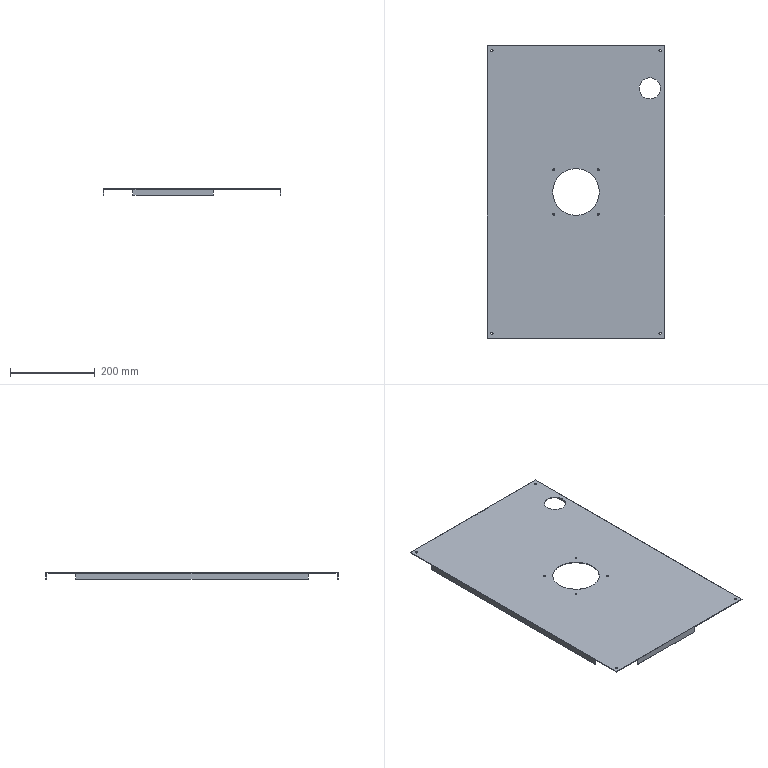Part | SolidWorks | features BaseBody 1 | 1 solid | 42 faces | box 418 x 688 x 15 mm | volume 443799 mm3 | plane 22 | cylinder 20 | commonest cylinder face diameters 4.2 x8 5.5 x8 50 x2 110 x2
STEP:
#1=CARTESIAN_POINT('',(49.25,332.999,-1.5));
#2=VERTEX_POINT('',#1);
#3=CARTESIAN_POINT('',(54.75,332.999,-1.5));
#4=VERTEX_POINT('',#3);
#5=CARTESIAN_POINT('',(52.,332.999,-1.5));
#6=DIRECTION('',(0.,0.,1.));
#7=DIRECTION('',(1.,0.,0.));
#8=AXIS2_PLACEMENT_3D('',#5,#6,#7);
#9=CIRCLE('',#8,2.75);
#10=EDGE_CURVE('',#2,#4,#9,.T.);
#11=ORIENTED_EDGE('',*,*,#10,.F.);
#12=CARTESIAN_POINT('',(49.25,332.999,0.));
#13=VERTEX_POINT('',#12);
#14=CARTESIAN_POINT('',(49.25,332.999,-15.));
#15=DIRECTION('',(0.,0.,1.));
#16=VECTOR('',#15,1000.);
#17=LINE('',#14,#16);
#18=EDGE_CURVE('',#2,#13,#17,.T.);
#19=ORIENTED_EDGE('',*,*,#18,.T.);
#20=CARTESIAN_POINT('',(54.75,332.999,0.));
#21=VERTEX_POINT('',#20);
#22=CARTESIAN_POINT('',(52.,332.999,0.));
#23=DIRECTION('',(0.,0.,-1.));
#24=DIRECTION('',(1.,0.,0.));
#25=AXIS2_PLACEMENT_3D('',#22,#23,#24);
#26=CIRCLE('',#25,2.75);
#27=EDGE_CURVE('',#21,#13,#26,.T.);
#28=ORIENTED_EDGE('',*,*,#27,.F.);
#29=CARTESIAN_POINT('',(54.75,332.999,-15.));
#30=DIRECTION('',(0.,0.,1.));
#31=VECTOR('',#30,1000.);
#32=LINE('',#29,#31);
#33=EDGE_CURVE('',#4,#21,#32,.T.);
#34=ORIENTED_EDGE('',*,*,#33,.F.);
#35=EDGE_LOOP('',(#11,#19,#28,#34));
#36=FACE_OUTER_BOUND('',#35,.T.);
#37=CARTESIAN_POINT('',(52.,332.999,-15.));
#38=DIRECTION('',(0.,0.,1.));
#39=DIRECTION('',(1.,0.,0.));
#40=AXIS2_PLACEMENT_3D('',#37,#38,#39);
#41=CYLINDRICAL_SURFACE('',#40,2.75);
#42=ADVANCED_FACE('',(#36),#41,.F.);
#43=CARTESIAN_POINT('',(445.249,333.,-1.5));
#44=VERTEX_POINT('',#43);
#45=CARTESIAN_POINT('',(450.749,333.,-1.5));
#46=VERTEX_POINT('',#45);
#47=CARTESIAN_POINT('',(447.999,333.,-1.5));
#48=DIRECTION('',(0.,0.,1.));
#49=DIRECTION('',(1.,0.,0.));
#50=AXIS2_PLACEMENT_3D('',#47,#48,#49);
#51=CIRCLE('',#50,2.75);
#52=EDGE_CURVE('',#44,#46,#51,.T.);
#53=ORIENTED_EDGE('',*,*,#52,.F.);
#54=CARTESIAN_POINT('',(445.249,333.,0.));
#55=VERTEX_POINT('',#54);
#56=CARTESIAN_POINT('',(445.249,333.,-15.));
#57=DIRECTION('',(0.,0.,1.));
#58=VECTOR('',#57,1000.);
#59=LINE('',#56,#58);
#60=EDGE_CURVE('',#44,#55,#59,.T.);
#61=ORIENTED_EDGE('',*,*,#60,.T.);
#62=CARTESIAN_POINT('',(450.749,333.,0.));
#63=VERTEX_POINT('',#62);
#64=CARTESIAN_POINT('',(447.999,333.,0.));
#65=DIRECTION('',(0.,0.,-1.));
#66=DIRECTION('',(1.,0.,0.));
#67=AXIS2_PLACEMENT_3D('',#64,#65,#66);
#68=CIRCLE('',#67,2.75);
#69=EDGE_CURVE('',#63,#55,#68,.T.);
#70=ORIENTED_EDGE('',*,*,#69,.F.);
#71=CARTESIAN_POINT('',(450.749,333.,-15.));
#72=DIRECTION('',(0.,0.,1.));
#73=VECTOR('',#72,1000.);
#74=LINE('',#71,#73);
#75=EDGE_CURVE('',#46,#63,#74,.T.);
#76=ORIENTED_EDGE('',*,*,#75,.F.);
#77=EDGE_LOOP('',(#53,#61,#70,#76));
#78=FACE_OUTER_BOUND('',#77,.T.);
#79=CARTESIAN_POINT('',(447.999,333.,-15.));
#80=DIRECTION('',(0.,0.,1.));
#81=DIRECTION('',(1.,0.,0.));
#82=AXIS2_PLACEMENT_3D('',#79,#80,#81);
#83=CYLINDRICAL_SURFACE('',#82,2.75);
#84=ADVANCED_FACE('',(#78),#83,.F.);
#85=CARTESIAN_POINT('',(49.251,-333.,-1.5));
#86=VERTEX_POINT('',#85);
#87=CARTESIAN_POINT('',(54.751,-333.,-1.5));
#88=VERTEX_POINT('',#87);
#89=CARTESIAN_POINT('',(52.001,-333.,-1.5));
#90=DIRECTION('',(0.,0.,1.));
#91=DIRECTION('',(1.,0.,0.));
#92=AXIS2_PLACEMENT_3D('',#89,#90,#91);
#93=CIRCLE('',#92,2.75);
#94=EDGE_CURVE('',#86,#88,#93,.T.);
#95=ORIENTED_EDGE('',*,*,#94,.F.);
#96=CARTESIAN_POINT('',(49.251,-333.,0.));
#97=VERTEX_POINT('',#96);
#98=CARTESIAN_POINT('',(49.251,-333.,-15.));
#99=DIRECTION('',(0.,0.,1.));
#100=VECTOR('',#99,1000.);
#101=LINE('',#98,#100);
#102=EDGE_CURVE('',#86,#97,#101,.T.);
#103=ORIENTED_EDGE('',*,*,#102,.T.);
#104=CARTESIAN_POINT('',(54.751,-333.,0.));
#105=VERTEX_POINT('',#104);
#106=CARTESIAN_POINT('',(52.001,-333.,0.));
#107=DIRECTION('',(0.,0.,-1.));
#108=DIRECTION('',(1.,0.,0.));
#109=AXIS2_PLACEMENT_3D('',#106,#107,#108);
#110=CIRCLE('',#109,2.75);
#111=EDGE_CURVE('',#105,#97,#110,.T.);
#112=ORIENTED_EDGE('',*,*,#111,.F.);
#113=CARTESIAN_POINT('',(54.751,-333.,-15.));
#114=DIRECTION('',(0.,0.,1.));
#115=VECTOR('',#114,1000.);
#116=LINE('',#113,#115);
#117=EDGE_CURVE('',#88,#105,#116,.T.);
#118=ORIENTED_EDGE('',*,*,#117,.F.);
#119=EDGE_LOOP('',(#95,#103,#112,#118));
#120=FACE_OUTER_BOUND('',#119,.T.);
#121=CARTESIAN_POINT('',(52.001,-333.,-15.));
#122=DIRECTION('',(0.,0.,1.));
#123=DIRECTION('',(1.,0.,0.));
#124=AXIS2_PLACEMENT_3D('',#121,#122,#123);
#125=CYLINDRICAL_SURFACE('',#124,2.75);
#126=ADVANCED_FACE('',(#120),#125,.F.);
#127=CARTESIAN_POINT('',(445.249,-333.,-1.5));
#128=VERTEX_POINT('',#127);
#129=CARTESIAN_POINT('',(450.749,-333.,-1.5));
#130=VERTEX_POINT('',#129);
#131=CARTESIAN_POINT('',(447.999,-333.,-1.5));
#132=DIRECTION('',(0.,0.,1.));
#133=DIRECTION('',(1.,0.,0.));
#134=AXIS2_PLACEMENT_3D('',#131,#132,#133);
#135=CIRCLE('',#134,2.75);
#136=EDGE_CURVE('',#128,#130,#135,.T.);
#137=ORIENTED_EDGE('',*,*,#136,.F.);
#138=CARTESIAN_POINT('',(445.249,-333.,0.));
#139=VERTEX_POINT('',#138);
#140=CARTESIAN_POINT('',(445.249,-333.,-15.));
#141=DIRECTION('',(0.,0.,1.));
#142=VECTOR('',#141,1000.);
#143=LINE('',#140,#142);
#144=EDGE_CURVE('',#128,#139,#143,.T.);
#145=ORIENTED_EDGE('',*,*,#144,.T.);
#146=CARTESIAN_POINT('',(450.749,-333.,0.));
#147=VERTEX_POINT('',#146);
#148=CARTESIAN_POINT('',(447.999,-333.,0.));
#149=DIRECTION('',(0.,0.,-1.));
#150=DIRECTION('',(1.,0.,0.));
#151=AXIS2_PLACEMENT_3D('',#148,#149,#150);
#152=CIRCLE('',#151,2.75);
#153=EDGE_CURVE('',#147,#139,#152,.T.);
#154=ORIENTED_EDGE('',*,*,#153,.F.);
#155=CARTESIAN_POINT('',(450.749,-333.,-15.));
#156=DIRECTION('',(0.,0.,1.));
#157=VECTOR('',#156,1000.);
#158=LINE('',#155,#157);
#159=EDGE_CURVE('',#130,#147,#158,.T.);
#160=ORIENTED_EDGE('',*,*,#159,.F.);
#161=EDGE_LOOP('',(#137,#145,#154,#160));
#162=FACE_OUTER_BOUND('',#161,.T.);
#163=CARTESIAN_POINT('',(447.999,-333.,-15.));
#164=DIRECTION('',(0.,0.,1.));
#165=DIRECTION('',(1.,0.,0.));
#166=AXIS2_PLACEMENT_3D('',#163,#164,#165);
#167=CYLINDRICAL_SURFACE('',#166,2.75);
#168=ADVANCED_FACE('',(#162),#167,.F.);
#169=CARTESIAN_POINT('',(399.,244.,-1.5));
#170=VERTEX_POINT('',#169);
#171=CARTESIAN_POINT('',(449.,244.,-1.5));
#172=VERTEX_POINT('',#171);
#173=CARTESIAN_POINT('',(424.,244.,-1.5));
#174=DIRECTION('',(0.,0.,1.));
#175=DIRECTION('',(1.,0.,0.));
#176=AXIS2_PLACEMENT_3D('',#173,#174,#175);
#177=CIRCLE('',#176,25.);
#178=EDGE_CURVE('',#170,#172,#177,.T.);
#179=ORIENTED_EDGE('',*,*,#178,.F.);
#180=CARTESIAN_POINT('',(399.,244.,0.));
#181=VERTEX_POINT('',#180);
#182=CARTESIAN_POINT('',(399.,244.,-15.));
#183=DIRECTION('',(0.,0.,1.));
#184=VECTOR('',#183,1000.);
#185=LINE('',#182,#184);
#186=EDGE_CURVE('',#170,#181,#185,.T.);
#187=ORIENTED_EDGE('',*,*,#186,.T.);
#188=CARTESIAN_POINT('',(449.,244.,0.));
#189=VERTEX_POINT('',#188);
#190=CARTESIAN_POINT('',(424.,244.,0.));
#191=DIRECTION('',(0.,0.,-1.));
#192=DIRECTION('',(1.,0.,0.));
#193=AXIS2_PLACEMENT_3D('',#190,#191,#192);
#194=CIRCLE('',#193,25.);
#195=EDGE_CURVE('',#189,#181,#194,.T.);
#196=ORIENTED_EDGE('',*,*,#195,.F.);
#197=CARTESIAN_POINT('',(449.,244.,-15.));
#198=DIRECTION('',(0.,0.,1.));
#199=VECTOR('',#198,1000.);
#200=LINE('',#197,#199);
#201=EDGE_CURVE('',#172,#189,#200,.T.);
#202=ORIENTED_EDGE('',*,*,#201,.F.);
#203=EDGE_LOOP('',(#179,#187,#196,#202));
#204=FACE_OUTER_BOUND('',#203,.T.);
#205=CARTESIAN_POINT('',(424.,244.,-15.));
#206=DIRECTION('',(0.,0.,1.));
#207=DIRECTION('',(1.,0.,0.));
#208=AXIS2_PLACEMENT_3D('',#205,#206,#207);
#209=CYLINDRICAL_SURFACE('',#208,25.);
#210=ADVANCED_FACE('',(#204),#209,.F.);
#211=CARTESIAN_POINT('',(195.,0.,-1.5));
#212=VERTEX_POINT('',#211);
#213=CARTESIAN_POINT('',(305.,0.,-1.5));
#214=VERTEX_POINT('',#213);
#215=CARTESIAN_POINT('',(250.,0.,-1.5));
#216=DIRECTION('',(0.,0.,1.));
#217=DIRECTION('',(1.,0.,0.));
#218=AXIS2_PLACEMENT_3D('',#215,#216,#217);
#219=CIRCLE('',#218,55.);
#220=EDGE_CURVE('',#212,#214,#219,.T.);
#221=ORIENTED_EDGE('',*,*,#220,.F.);
#222=CARTESIAN_POINT('',(195.,0.,0.));
#223=VERTEX_POINT('',#222);
#224=CARTESIAN_POINT('',(195.,0.,-15.001));
#225=DIRECTION('',(0.,0.,1.));
#226=VECTOR('',#225,1000.);
#227=LINE('',#224,#226);
#228=EDGE_CURVE('',#212,#223,#227,.T.);
#229=ORIENTED_EDGE('',*,*,#228,.T.);
#230=CARTESIAN_POINT('',(305.,0.,0.));
#231=VERTEX_POINT('',#230);
#232=CARTESIAN_POINT('',(250.,0.,0.));
#233=DIRECTION('',(0.,0.,-1.));
#234=DIRECTION('',(1.,0.,0.));
#235=AXIS2_PLACEMENT_3D('',#232,#233,#234);
#236=CIRCLE('',#235,55.);
#237=EDGE_CURVE('',#231,#223,#236,.T.);
#238=ORIENTED_EDGE('',*,*,#237,.F.);
#239=CARTESIAN_POINT('',(305.,0.,-15.001));
#240=DIRECTION('',(0.,0.,1.));
#241=VECTOR('',#240,1000.);
#242=LINE('',#239,#241);
#243=EDGE_CURVE('',#214,#231,#242,.T.);
#244=ORIENTED_EDGE('',*,*,#243,.F.);
#245=EDGE_LOOP('',(#221,#229,#238,#244));
#246=FACE_OUTER_BOUND('',#245,.T.);
#247=CARTESIAN_POINT('',(250.,0.,-15.001));
#248=DIRECTION('',(0.,0.,1.));
#249=DIRECTION('',(1.,0.,0.));
#250=AXIS2_PLACEMENT_3D('',#247,#248,#249);
#251=CYLINDRICAL_SURFACE('',#250,55.);
#252=ADVANCED_FACE('',(#246),#251,.F.);
#253=CARTESIAN_POINT('',(304.6,-52.5,0.));
#254=VERTEX_POINT('',#253);
#255=CARTESIAN_POINT('',(300.4,-52.5,0.));
#256=VERTEX_POINT('',#255);
#257=CARTESIAN_POINT('',(302.5,-52.5,0.));
#258=DIRECTION('',(0.,0.,-1.));
#259=DIRECTION('',(-1.,0.,0.));
#260=AXIS2_PLACEMENT_3D('',#257,#258,#259);
#261=CIRCLE('',#260,2.1);
#262=EDGE_CURVE('',#254,#256,#261,.T.);
#263=ORIENTED_EDGE('',*,*,#262,.F.);
#264=CARTESIAN_POINT('',(304.6,-52.5,-1.5));
#265=VERTEX_POINT('',#264);
#266=CARTESIAN_POINT('',(304.6,-52.5,-1.5));
#267=DIRECTION('',(0.,0.,-1.));
#268=VECTOR('',#267,1000.);
#269=LINE('',#266,#268);
#270=EDGE_CURVE('',#254,#265,#269,.T.);
#271=ORIENTED_EDGE('',*,*,#270,.T.);
#272=CARTESIAN_POINT('',(300.4,-52.5,-1.5));
#273=VERTEX_POINT('',#272);
#274=CARTESIAN_POINT('',(302.5,-52.5,-1.5));
#275=DIRECTION('',(0.,0.,1.));
#276=DIRECTION('',(-1.,0.,0.));
#277=AXIS2_PLACEMENT_3D('',#274,#275,#276);
#278=CIRCLE('',#277,2.1);
#279=EDGE_CURVE('',#273,#265,#278,.T.);
#280=ORIENTED_EDGE('',*,*,#279,.F.);
#281=CARTESIAN_POINT('',(300.4,-52.5,-1.5));
#282=DIRECTION('',(0.,0.,-1.));
#283=VECTOR('',#282,1000.);
#284=LINE('',#281,#283);
#285=EDGE_CURVE('',#256,#273,#284,.T.);
#286=ORIENTED_EDGE('',*,*,#285,.F.);
#287=EDGE_LOOP('',(#263,#271,#280,#286));
#288=FACE_OUTER_BOUND('',#287,.T.);
#289=CARTESIAN_POINT('',(302.5,-52.5,-1.5));
#290=DIRECTION('',(0.,0.,-1.));
#291=DIRECTION('',(-1.,0.,0.));
#292=AXIS2_PLACEMENT_3D('',#289,#290,#291);
#293=CYLINDRICAL_SURFACE('',#292,2.1);
#294=ADVANCED_FACE('',(#288),#293,.F.);
#295=CARTESIAN_POINT('',(199.6,-52.5,0.));
#296=VERTEX_POINT('',#295);
#297=CARTESIAN_POINT('',(195.4,-52.5,0.));
#298=VERTEX_POINT('',#297);
#299=CARTESIAN_POINT('',(197.5,-52.5,0.));
#300=DIRECTION('',(0.,0.,-1.));
#301=DIRECTION('',(-1.,0.,0.));
#302=AXIS2_PLACEMENT_3D('',#299,#300,#301);
#303=CIRCLE('',#302,2.1);
#304=EDGE_CURVE('',#296,#298,#303,.T.);
#305=ORIENTED_EDGE('',*,*,#304,.F.);
#306=CARTESIAN_POINT('',(199.6,-52.5,-1.5));
#307=VERTEX_POINT('',#306);
#308=CARTESIAN_POINT('',(199.6,-52.5,-1.5));
#309=DIRECTION('',(0.,0.,-1.));
#310=VECTOR('',#309,1000.);
#311=LINE('',#308,#310);
#312=EDGE_CURVE('',#296,#307,#311,.T.);
#313=ORIENTED_EDGE('',*,*,#312,.T.);
#314=CARTESIAN_POINT('',(195.4,-52.5,-1.5));
#315=VERTEX_POINT('',#314);
#316=CARTESIAN_POINT('',(197.5,-52.5,-1.5));
#317=DIRECTION('',(0.,0.,1.));
#318=DIRECTION('',(-1.,0.,0.));
#319=AXIS2_PLACEMENT_3D('',#316,#317,#318);
#320=CIRCLE('',#319,2.1);
#321=EDGE_CURVE('',#315,#307,#320,.T.);
#322=ORIENTED_EDGE('',*,*,#321,.F.);
#323=CARTESIAN_POINT('',(195.4,-52.5,-1.5));
#324=DIRECTION('',(0.,0.,-1.));
#325=VECTOR('',#324,1000.);
#326=LINE('',#323,#325);
#327=EDGE_CURVE('',#298,#315,#326,.T.);
#328=ORIENTED_EDGE('',*,*,#327,.F.);
#329=EDGE_LOOP('',(#305,#313,#322,#328));
#330=FACE_OUTER_BOUND('',#329,.T.);
#331=CARTESIAN_POINT('',(197.5,-52.5,-1.5));
#332=DIRECTION('',(0.,0.,-1.));
#333=DIRECTION('',(-1.,0.,0.));
#334=AXIS2_PLACEMENT_3D('',#331,#332,#333);
#335=CYLINDRICAL_SURFACE('',#334,2.1);
#336=ADVANCED_FACE('',(#330),#335,.F.);
#337=CARTESIAN_POINT('',(199.6,52.5,0.));
#338=VERTEX_POINT('',#337);
#339=CARTESIAN_POINT('',(195.4,52.5,0.));
#340=VERTEX_POINT('',#339);
#341=CARTESIAN_POINT('',(197.5,52.5,0.));
#342=DIRECTION('',(0.,0.,-1.));
#343=DIRECTION('',(-1.,0.,0.));
#344=AXIS2_PLACEMENT_3D('',#341,#342,#343);
#345=CIRCLE('',#344,2.1);
#346=EDGE_CURVE('',#338,#340,#345,.T.);
#347=ORIENTED_EDGE('',*,*,#346,.F.);
#348=CARTESIAN_POINT('',(199.6,52.5,-1.5));
#349=VERTEX_POINT('',#348);
#350=CARTESIAN_POINT('',(199.6,52.5,-1.5));
#351=DIRECTION('',(0.,0.,-1.));
#352=VECTOR('',#351,1000.);
#353=LINE('',#350,#352);
#354=EDGE_CURVE('',#338,#349,#353,.T.);
#355=ORIENTED_EDGE('',*,*,#354,.T.);
#356=CARTESIAN_POINT('',(195.4,52.5,-1.5));
#357=VERTEX_POINT('',#356);
#358=CARTESIAN_POINT('',(197.5,52.5,-1.5));
#359=DIRECTION('',(0.,0.,1.));
#360=DIRECTION('',(-1.,0.,0.));
#361=AXIS2_PLACEMENT_3D('',#358,#359,#360);
#362=CIRCLE('',#361,2.1);
#363=EDGE_CURVE('',#357,#349,#362,.T.);
#364=ORIENTED_EDGE('',*,*,#363,.F.);
#365=CARTESIAN_POINT('',(195.4,52.5,-1.5));
#366=DIRECTION('',(0.,0.,-1.));
#367=VECTOR('',#366,1000.);
#368=LINE('',#365,#367);
#369=EDGE_CURVE('',#340,#357,#368,.T.);
#370=ORIENTED_EDGE('',*,*,#369,.F.);
#371=EDGE_LOOP('',(#347,#355,#364,#370));
#372=FACE_OUTER_BOUND('',#371,.T.);
#373=CARTESIAN_POINT('',(197.5,52.5,-1.5));
#374=DIRECTION('',(0.,0.,-1.));
#375=DIRECTION('',(-1.,0.,0.));
#376=AXIS2_PLACEMENT_3D('',#373,#374,#375);
#377=CYLINDRICAL_SURFACE('',#376,2.1);
#378=ADVANCED_FACE('',(#372),#377,.F.);
#379=CARTESIAN_POINT('',(304.6,52.5,0.));
#380=VERTEX_POINT('',#379);
#381=CARTESIAN_POINT('',(300.4,52.5,0.));
#382=VERTEX_POINT('',#381);
#383=CARTESIAN_POINT('',(302.5,52.5,0.));
#384=DIRECTION('',(0.,0.,-1.));
#385=DIRECTION('',(-1.,0.,0.));
#386=AXIS2_PLACEMENT_3D('',#383,#384,#385);
#387=CIRCLE('',#386,2.1);
#388=EDGE_CURVE('',#380,#382,#387,.T.);
#389=ORIENTED_EDGE('',*,*,#388,.F.);
#390=CARTESIAN_POINT('',(304.6,52.5,-1.5));
#391=VERTEX_POINT('',#390);
#392=CARTESIAN_POINT('',(304.6,52.5,-1.5));
#393=DIRECTION('',(0.,0.,-1.));
#394=VECTOR('',#393,1000.);
#395=LINE('',#392,#394);
#396=EDGE_CURVE('',#380,#391,#395,.T.);
#397=ORIENTED_EDGE('',*,*,#396,.T.);
#398=CARTESIAN_POINT('',(300.4,52.5,-1.5));
#399=VERTEX_POINT('',#398);
#400=CARTESIAN_POINT('',(302.5,52.5,-1.5));
#401=DIRECTION('',(0.,0.,1.));
#402=DIRECTION('',(-1.,0.,0.));
#403=AXIS2_PLACEMENT_3D('',#400,#401,#402);
#404=CIRCLE('',#403,2.1);
#405=EDGE_CURVE('',#399,#391,#404,.T.);
#406=ORIENTED_EDGE('',*,*,#405,.F.);
#407=CARTESIAN_POINT('',(300.4,52.5,-1.5));
#408=DIRECTION('',(0.,0.,-1.));
#409=VECTOR('',#408,1000.);
#410=LINE('',#407,#409);
#411=EDGE_CURVE('',#382,#399,#410,.T.);
#412=ORIENTED_EDGE('',*,*,#411,.F.);
#413=EDGE_LOOP('',(#389,#397,#406,#412));
#414=FACE_OUTER_BOUND('',#413,.T.);
#415=CARTESIAN_POINT('',(302.5,52.5,-1.5));
#416=DIRECTION('',(0.,0.,-1.));
#417=DIRECTION('',(-1.,0.,0.));
#418=AXIS2_PLACEMENT_3D('',#415,#416,#417);
#419=CYLINDRICAL_SURFACE('',#418,2.1);
#420=ADVANCED_FACE('',(#414),#419,.F.);
#421=CARTESIAN_POINT('',(459.,-344.,0.));
#422=VERTEX_POINT('',#421);
#423=CARTESIAN_POINT('',(459.,344.,0.));
#424=VERTEX_POINT('',#423);
#425=CARTESIAN_POINT('',(459.,0.,0.));
#426=DIRECTION('',(0.,1.,0.));
#427=VECTOR('',#426,1000.);
#428=LINE('',#425,#427);
#429=EDGE_CURVE('',#422,#424,#428,.T.);
#430=ORIENTED_EDGE('',*,*,#429,.T.);
#431=CARTESIAN_POINT('',(41.,344.,0.));
#432=VERTEX_POINT('',#431);
#433=CARTESIAN_POINT('',(0.,344.,0.));
#434=DIRECTION('',(-1.,0.,0.));
#435=VECTOR('',#434,1000.);
#436=LINE('',#433,#435);
#437=EDGE_CURVE('',#424,#432,#436,.T.);
#438=ORIENTED_EDGE('',*,*,#437,.T.);
#439=CARTESIAN_POINT('',(41.,-344.,0.));
#440=VERTEX_POINT('',#439);
#441=CARTESIAN_POINT('',(41.,0.,0.));
#442=DIRECTION('',(0.,-1.,0.));
#443=VECTOR('',#442,1000.);
#444=LINE('',#441,#443);
#445=EDGE_CURVE('',#432,#440,#444,.T.);
#446=ORIENTED_EDGE('',*,*,#445,.T.);
#447=CARTESIAN_POINT('',(0.,-344.,0.));
#448=DIRECTION('',(1.,0.,0.));
#449=VECTOR('',#448,1000.);
#450=LINE('',#447,#449);
#451=EDGE_CURVE('',#440,#422,#450,.T.);
#452=ORIENTED_EDGE('',*,*,#451,.T.);
#453=EDGE_LOOP('',(#430,#438,#446,#452));
#454=FACE_OUTER_BOUND('',#453,.T.);
#455=ORIENTED_EDGE('',*,*,#27,.T.);
#456=CARTESIAN_POINT('',(52.,332.999,0.));
#457=DIRECTION('',(0.,0.,-1.));
#458=DIRECTION('',(1.,0.,0.));
#459=AXIS2_PLACEMENT_3D('',#456,#457,#458);
#460=CIRCLE('',#459,2.75);
#461=EDGE_CURVE('',#13,#21,#460,.T.);
#462=ORIENTED_EDGE('',*,*,#461,.T.);
#463=EDGE_LOOP('',(#455,#462));
#464=FACE_BOUND('',#463,.T.);
#465=ORIENTED_EDGE('',*,*,#69,.T.);
#466=CARTESIAN_POINT('',(447.999,333.,0.));
#467=DIRECTION('',(0.,0.,-1.));
#468=DIRECTION('',(1.,0.,0.));
#469=AXIS2_PLACEMENT_3D('',#466,#467,#468);
#470=CIRCLE('',#469,2.75);
#471=EDGE_CURVE('',#55,#63,#470,.T.);
#472=ORIENTED_EDGE('',*,*,#471,.T.);
#473=EDGE_LOOP('',(#465,#472));
#474=FACE_BOUND('',#473,.T.);
#475=ORIENTED_EDGE('',*,*,#111,.T.);
#476=CARTESIAN_POINT('',(52.001,-333.,0.));
#477=DIRECTION('',(0.,0.,-1.));
#478=DIRECTION('',(1.,0.,0.));
#479=AXIS2_PLACEMENT_3D('',#476,#477,#478);
#480=CIRCLE('',#479,2.75);
#481=EDGE_CURVE('',#97,#105,#480,.T.);
#482=ORIENTED_EDGE('',*,*,#481,.T.);
#483=EDGE_LOOP('',(#475,#482));
#484=FACE_BOUND('',#483,.T.);
#485=ORIENTED_EDGE('',*,*,#153,.T.);
#486=CARTESIAN_POINT('',(447.999,-333.,0.));
#487=DIRECTION('',(0.,0.,-1.));
#488=DIRECTION('',(1.,0.,0.));
#489=AXIS2_PLACEMENT_3D('',#486,#487,#488);
#490=CIRCLE('',#489,2.75);
#491=EDGE_CURVE('',#139,#147,#490,.T.);
#492=ORIENTED_EDGE('',*,*,#491,.T.);
#493=EDGE_LOOP('',(#485,#492));
#494=FACE_BOUND('',#493,.T.);
#495=ORIENTED_EDGE('',*,*,#195,.T.);
#496=CARTESIAN_POINT('',(424.,244.,0.));
#497=DIRECTION('',(0.,0.,-1.));
#498=DIRECTION('',(1.,0.,0.));
#499=AXIS2_PLACEMENT_3D('',#496,#497,#498);
#500=CIRCLE('',#499,25.);
#501=EDGE_CURVE('',#181,#189,#500,.T.);
#502=ORIENTED_EDGE('',*,*,#501,.T.);
#503=EDGE_LOOP('',(#495,#502));
#504=FACE_BOUND('',#503,.T.);
#505=ORIENTED_EDGE('',*,*,#237,.T.);
#506=CARTESIAN_POINT('',(250.,0.,0.));
#507=DIRECTION('',(0.,0.,-1.));
#508=DIRECTION('',(1.,0.,0.));
#509=AXIS2_PLACEMENT_3D('',#506,#507,#508);
#510=CIRCLE('',#509,55.);
#511=EDGE_CURVE('',#223,#231,#510,.T.);
#512=ORIENTED_EDGE('',*,*,#511,.T.);
#513=EDGE_LOOP('',(#505,#512));
#514=FACE_BOUND('',#513,.T.);
#515=CARTESIAN_POINT('',(302.5,-52.5,0.));
#516=DIRECTION('',(0.,0.,-1.));
#517=DIRECTION('',(-1.,0.,0.));
#518=AXIS2_PLACEMENT_3D('',#515,#516,#517);
#519=CIRCLE('',#518,2.1);
#520=EDGE_CURVE('',#256,#254,#519,.T.);
#521=ORIENTED_EDGE('',*,*,#520,.T.);
#522=ORIENTED_EDGE('',*,*,#262,.T.);
#523=EDGE_LOOP('',(#521,#522));
#524=FACE_BOUND('',#523,.T.);
#525=CARTESIAN_POINT('',(197.5,-52.5,0.));
#526=DIRECTION('',(0.,0.,-1.));
#527=DIRECTION('',(-1.,0.,0.));
#528=AXIS2_PLACEMENT_3D('',#525,#526,#527);
#529=CIRCLE('',#528,2.1);
#530=EDGE_CURVE('',#298,#296,#529,.T.);
#531=ORIENTED_EDGE('',*,*,#530,.T.);
#532=ORIENTED_EDGE('',*,*,#304,.T.);
#533=EDGE_LOOP('',(#531,#532));
#534=FACE_BOUND('',#533,.T.);
#535=CARTESIAN_POINT('',(197.5,52.5,0.));
#536=DIRECTION('',(0.,0.,-1.));
#537=DIRECTION('',(-1.,0.,0.));
#538=AXIS2_PLACEMENT_3D('',#535,#536,#537);
#539=CIRCLE('',#538,2.1);
#540=EDGE_CURVE('',#340,#338,#539,.T.);
#541=ORIENTED_EDGE('',*,*,#540,.T.);
#542=ORIENTED_EDGE('',*,*,#346,.T.);
#543=EDGE_LOOP('',(#541,#542));
#544=FACE_BOUND('',#543,.T.);
#545=CARTESIAN_POINT('',(302.5,52.5,0.));
#546=DIRECTION('',(0.,0.,-1.));
#547=DIRECTION('',(-1.,0.,0.));
#548=AXIS2_PLACEMENT_3D('',#545,#546,#547);
#549=CIRCLE('',#548,2.1);
#550=EDGE_CURVE('',#382,#380,#549,.T.);
#551=ORIENTED_EDGE('',*,*,#550,.T.);
#552=ORIENTED_EDGE('',*,*,#388,.T.);
#553=EDGE_LOOP('',(#551,#552));
#554=FACE_BOUND('',#553,.T.);
#555=CARTESIAN_POINT('',(0.,0.,0.));
#556=DIRECTION('',(0.,0.,1.));
#557=DIRECTION('',(1.,0.,0.));
#558=AXIS2_PLACEMENT_3D('',#555,#556,#557);
#559=PLANE('',#558);
#560=ADVANCED_FACE('',(#454,#464,#474,#484,#494,#504,#514,#524,#534,#544,#554),#559,.T.);
#561=ORIENTED_EDGE('',*,*,#437,.F.);
#562=CARTESIAN_POINT('',(459.,344.,-1.5));
#563=VERTEX_POINT('',#562);
#564=CARTESIAN_POINT('',(459.,344.,-15.));
#565=DIRECTION('',(0.,0.,-1.));
#566=VECTOR('',#565,1000.);
#567=LINE('',#564,#566);
#568=EDGE_CURVE('',#424,#563,#567,.T.);
#569=ORIENTED_EDGE('',*,*,#568,.T.);
#570=CARTESIAN_POINT('',(300.,344.,-1.5));
#571=VERTEX_POINT('',#570);
#572=CARTESIAN_POINT('',(41.,344.,-1.5));
#573=DIRECTION('',(-1.,0.,0.));
#574=VECTOR('',#573,1000.);
#575=LINE('',#572,#574);
#576=EDGE_CURVE('',#563,#571,#575,.T.);
#577=ORIENTED_EDGE('',*,*,#576,.T.);
#578=CARTESIAN_POINT('',(300.,344.,-15.));
#579=VERTEX_POINT('',#578);
#580=CARTESIAN_POINT('',(300.,344.,-15.));
#581=DIRECTION('',(0.,0.,-1.));
#582=VECTOR('',#581,1000.);
#583=LINE('',#580,#582);
#584=EDGE_CURVE('',#571,#579,#583,.T.);
#585=ORIENTED_EDGE('',*,*,#584,.T.);
#586=CARTESIAN_POINT('',(111.,344.,-15.));
#587=VERTEX_POINT('',#586);
#588=CARTESIAN_POINT('',(41.,344.,-15.));
#589=DIRECTION('',(-1.,0.,0.));
#590=VECTOR('',#589,1000.);
#591=LINE('',#588,#590);
#592=EDGE_CURVE('',#579,#587,#591,.T.);
#593=ORIENTED_EDGE('',*,*,#592,.T.);
#594=CARTESIAN_POINT('',(111.,344.,-1.5));
#595=VERTEX_POINT('',#594);
#596=CARTESIAN_POINT('',(111.,344.,-15.));
#597=DIRECTION('',(0.,0.,1.));
#598=VECTOR('',#597,1000.);
#599=LINE('',#596,#598);
#600=EDGE_CURVE('',#587,#595,#599,.T.);
#601=ORIENTED_EDGE('',*,*,#600,.T.);
#602=CARTESIAN_POINT('',(41.,344.,-1.5));
#603=VERTEX_POINT('',#602);
#604=CARTESIAN_POINT('',(41.,344.,-1.5));
#605=DIRECTION('',(-1.,0.,0.));
#606=VECTOR('',#605,1000.);
#607=LINE('',#604,#606);
#608=EDGE_CURVE('',#595,#603,#607,.T.);
#609=ORIENTED_EDGE('',*,*,#608,.T.);
#610=CARTESIAN_POINT('',(41.,344.,-15.));
#611=DIRECTION('',(0.,0.,1.));
#612=VECTOR('',#611,1000.);
#613=LINE('',#610,#612);
#614=EDGE_CURVE('',#603,#432,#613,.T.);
#615=ORIENTED_EDGE('',*,*,#614,.T.);
#616=EDGE_LOOP('',(#561,#569,#577,#585,#593,#601,#609,#615));
#617=FACE_OUTER_BOUND('',#616,.T.);
#618=CARTESIAN_POINT('',(41.,344.,-15.));
#619=DIRECTION('',(0.,1.,0.));
#620=DIRECTION('',(0.,0.,1.));
#621=AXIS2_PLACEMENT_3D('',#618,#619,#620);
#622=PLANE('',#621);
#623=ADVANCED_FACE('',(#617),#622,.T.);
#624=ORIENTED_EDGE('',*,*,#429,.F.);
#625=CARTESIAN_POINT('',(459.,-344.,-1.5));
#626=VERTEX_POINT('',#625);
#627=CARTESIAN_POINT('',(459.,-344.,-15.));
#628=DIRECTION('',(0.,0.,-1.));
#629=VECTOR('',#628,1000.);
#630=LINE('',#627,#629);
#631=EDGE_CURVE('',#422,#626,#630,.T.);
#632=ORIENTED_EDGE('',*,*,#631,.T.);
#633=CARTESIAN_POINT('',(459.,-274.,-1.5));
#634=VERTEX_POINT('',#633);
#635=CARTESIAN_POINT('',(459.,344.,-1.5));
#636=DIRECTION('',(0.,1.,0.));
#637=VECTOR('',#636,1000.);
#638=LINE('',#635,#637);
#639=EDGE_CURVE('',#626,#634,#638,.T.);
#640=ORIENTED_EDGE('',*,*,#639,.T.);
#641=CARTESIAN_POINT('',(459.,-274.,-15.));
#642=VERTEX_POINT('',#641);
#643=CARTESIAN_POINT('',(459.,-274.,-15.));
#644=DIRECTION('',(0.,0.,-1.));
#645=VECTOR('',#644,1000.);
#646=LINE('',#643,#645);
#647=EDGE_CURVE('',#634,#642,#646,.T.);
#648=ORIENTED_EDGE('',*,*,#647,.T.);
#649=CARTESIAN_POINT('',(459.,274.,-15.));
#650=VERTEX_POINT('',#649);
#651=CARTESIAN_POINT('',(459.,344.,-15.));
#652=DIRECTION('',(0.,1.,0.));
#653=VECTOR('',#652,1000.);
#654=LINE('',#651,#653);
#655=EDGE_CURVE('',#642,#650,#654,.T.);
#656=ORIENTED_EDGE('',*,*,#655,.T.);
#657=CARTESIAN_POINT('',(459.,274.,-1.5));
#658=VERTEX_POINT('',#657);
#659=CARTESIAN_POINT('',(459.,274.,-15.));
#660=DIRECTION('',(0.,0.,1.));
#661=VECTOR('',#660,1000.);
#662=LINE('',#659,#661);
#663=EDGE_CURVE('',#650,#658,#662,.T.);
#664=ORIENTED_EDGE('',*,*,#663,.T.);
#665=CARTESIAN_POINT('',(459.,344.,-1.5));
#666=DIRECTION('',(0.,1.,0.));
#667=VECTOR('',#666,1000.);
#668=LINE('',#665,#667);
#669=EDGE_CURVE('',#658,#563,#668,.T.);
#670=ORIENTED_EDGE('',*,*,#669,.T.);
#671=ORIENTED_EDGE('',*,*,#568,.F.);
#672=EDGE_LOOP('',(#624,#632,#640,#648,#656,#664,#670,#671));
#673=FACE_OUTER_BOUND('',#672,.T.);
#674=CARTESIAN_POINT('',(459.,344.,-15.));
#675=DIRECTION('',(1.,0.,0.));
#676=DIRECTION('',(0.,1.,0.));
#677=AXIS2_PLACEMENT_3D('',#674,#675,#676);
#678=PLANE('',#677);
#679=ADVANCED_FACE('',(#673),#678,.T.);
#680=CARTESIAN_POINT('',(41.,-344.,-1.5));
#681=VERTEX_POINT('',#680);
#682=CARTESIAN_POINT('',(111.,-344.,-1.5));
#683=VERTEX_POINT('',#682);
#684=CARTESIAN_POINT('',(41.,-344.,-1.5));
#685=DIRECTION('',(1.,0.,0.));
#686=VECTOR('',#685,1000.);
#687=LINE('',#684,#686);
#688=EDGE_CURVE('',#681,#683,#687,.T.);
#689=ORIENTED_EDGE('',*,*,#688,.T.);
#690=CARTESIAN_POINT('',(111.,-344.,-15.));
#691=VERTEX_POINT('',#690);
#692=CARTESIAN_POINT('',(111.,-344.,-15.));
#693=DIRECTION('',(0.,0.,-1.));
#694=VECTOR('',#693,1000.);
#695=LINE('',#692,#694);
#696=EDGE_CURVE('',#683,#691,#695,.T.);
#697=ORIENTED_EDGE('',*,*,#696,.T.);
#698=CARTESIAN_POINT('',(300.,-344.,-15.));
#699=VERTEX_POINT('',#698);
#700=CARTESIAN_POINT('',(41.,-344.,-15.));
#701=DIRECTION('',(1.,0.,0.));
#702=VECTOR('',#701,1000.);
#703=LINE('',#700,#702);
#704=EDGE_CURVE('',#691,#699,#703,.T.);
#705=ORIENTED_EDGE('',*,*,#704,.T.);
#706=CARTESIAN_POINT('',(300.,-344.,-1.5));
#707=VERTEX_POINT('',#706);
#708=CARTESIAN_POINT('',(300.,-344.,-15.));
#709=DIRECTION('',(0.,0.,1.));
#710=VECTOR('',#709,1000.);
#711=LINE('',#708,#710);
#712=EDGE_CURVE('',#699,#707,#711,.T.);
#713=ORIENTED_EDGE('',*,*,#712,.T.);
#714=CARTESIAN_POINT('',(41.,-344.,-1.5));
#715=DIRECTION('',(1.,0.,0.));
#716=VECTOR('',#715,1000.);
#717=LINE('',#714,#716);
#718=EDGE_CURVE('',#707,#626,#717,.T.);
#719=ORIENTED_EDGE('',*,*,#718,.T.);
#720=ORIENTED_EDGE('',*,*,#631,.F.);
#721=ORIENTED_EDGE('',*,*,#451,.F.);
#722=CARTESIAN_POINT('',(41.,-344.,-15.));
#723=DIRECTION('',(0.,0.,-1.));
#724=VECTOR('',#723,1000.);
#725=LINE('',#722,#724);
#726=EDGE_CURVE('',#440,#681,#725,.T.);
#727=ORIENTED_EDGE('',*,*,#726,.T.);
#728=EDGE_LOOP('',(#689,#697,#705,#713,#719,#720,#721,#727));
#729=FACE_OUTER_BOUND('',#728,.T.);
#730=CARTESIAN_POINT('',(41.,-344.,-15.));
#731=DIRECTION('',(0.,-1.,0.));
#732=DIRECTION('',(0.,0.,-1.));
#733=AXIS2_PLACEMENT_3D('',#730,#731,#732);
#734=PLANE('',#733);
#735=ADVANCED_FACE('',(#729),#734,.T.);
#736=CARTESIAN_POINT('',(41.,274.,-1.5));
#737=VERTEX_POINT('',#736);
#738=CARTESIAN_POINT('',(41.,344.,-1.5));
#739=DIRECTION('',(0.,-1.,0.));
#740=VECTOR('',#739,1000.);
#741=LINE('',#738,#740);
#742=EDGE_CURVE('',#603,#737,#741,.T.);
#743=ORIENTED_EDGE('',*,*,#742,.T.);
#744=CARTESIAN_POINT('',(41.,274.,-15.));
#745=VERTEX_POINT('',#744);
#746=CARTESIAN_POINT('',(41.,274.,-15.));
#747=DIRECTION('',(0.,0.,-1.));
#748=VECTOR('',#747,1000.);
#749=LINE('',#746,#748);
#750=EDGE_CURVE('',#737,#745,#749,.T.);
#751=ORIENTED_EDGE('',*,*,#750,.T.);
#752=CARTESIAN_POINT('',(41.,-274.,-15.));
#753=VERTEX_POINT('',#752);
#754=CARTESIAN_POINT('',(41.,344.,-15.));
#755=DIRECTION('',(0.,-1.,0.));
#756=VECTOR('',#755,1000.);
#757=LINE('',#754,#756);
#758=EDGE_CURVE('',#745,#753,#757,.T.);
#759=ORIENTED_EDGE('',*,*,#758,.T.);
#760=CARTESIAN_POINT('',(41.,-274.,-1.5));
#761=VERTEX_POINT('',#760);
#762=CARTESIAN_POINT('',(41.,-274.,-15.));
#763=DIRECTION('',(0.,0.,1.));
#764=VECTOR('',#763,1000.);
#765=LINE('',#762,#764);
#766=EDGE_CURVE('',#753,#761,#765,.T.);
#767=ORIENTED_EDGE('',*,*,#766,.T.);
#768=CARTESIAN_POINT('',(41.,344.,-1.5));
#769=DIRECTION('',(0.,-1.,0.));
#770=VECTOR('',#769,1000.);
#771=LINE('',#768,#770);
#772=EDGE_CURVE('',#761,#681,#771,.T.);
#773=ORIENTED_EDGE('',*,*,#772,.T.);
#774=ORIENTED_EDGE('',*,*,#726,.F.);
#775=ORIENTED_EDGE('',*,*,#445,.F.);
#776=ORIENTED_EDGE('',*,*,#614,.F.);
#777=EDGE_LOOP('',(#743,#751,#759,#767,#773,#774,#775,#776));
#778=FACE_OUTER_BOUND('',#777,.T.);
#779=CARTESIAN_POINT('',(41.,344.,-15.));
#780=DIRECTION('',(-1.,0.,0.));
#781=DIRECTION('',(0.,-1.,0.));
#782=AXIS2_PLACEMENT_3D('',#779,#780,#781);
#783=PLANE('',#782);
#784=ADVANCED_FACE('',(#778),#783,.T.);
#785=ORIENTED_EDGE('',*,*,#18,.F.);
#786=CARTESIAN_POINT('',(52.,332.999,-1.5));
#787=DIRECTION('',(0.,0.,1.));
#788=DIRECTION('',(1.,0.,0.));
#789=AXIS2_PLACEMENT_3D('',#786,#787,#788);
#790=CIRCLE('',#789,2.75);
#791=EDGE_CURVE('',#4,#2,#790,.T.);
#792=ORIENTED_EDGE('',*,*,#791,.F.);
#793=ORIENTED_EDGE('',*,*,#33,.T.);
#794=ORIENTED_EDGE('',*,*,#461,.F.);
#795=EDGE_LOOP('',(#785,#792,#793,#794));
#796=FACE_OUTER_BOUND('',#795,.T.);
#797=CARTESIAN_POINT('',(52.,332.999,-15.));
#798=DIRECTION('',(0.,0.,1.));
#799=DIRECTION('',(1.,0.,0.));
#800=AXIS2_PLACEMENT_3D('',#797,#798,#799);
#801=CYLINDRICAL_SURFACE('',#800,2.75);
#802=ADVANCED_FACE('',(#796),#801,.F.);
#803=ORIENTED_EDGE('',*,*,#60,.F.);
#804=CARTESIAN_POINT('',(447.999,333.,-1.5));
#805=DIRECTION('',(0.,0.,1.));
#806=DIRECTION('',(1.,0.,0.));
#807=AXIS2_PLACEMENT_3D('',#804,#805,#806);
#808=CIRCLE('',#807,2.75);
#809=EDGE_CURVE('',#46,#44,#808,.T.);
#810=ORIENTED_EDGE('',*,*,#809,.F.);
#811=ORIENTED_EDGE('',*,*,#75,.T.);
#812=ORIENTED_EDGE('',*,*,#471,.F.);
#813=EDGE_LOOP('',(#803,#810,#811,#812));
#814=FACE_OUTER_BOUND('',#813,.T.);
#815=CARTESIAN_POINT('',(447.999,333.,-15.));
#816=DIRECTION('',(0.,0.,1.));
#817=DIRECTION('',(1.,0.,0.));
#818=AXIS2_PLACEMENT_3D('',#815,#816,#817);
#819=CYLINDRICAL_SURFACE('',#818,2.75);
#820=ADVANCED_FACE('',(#814),#819,.F.);
#821=ORIENTED_EDGE('',*,*,#102,.F.);
#822=CARTESIAN_POINT('',(52.001,-333.,-1.5));
#823=DIRECTION('',(0.,0.,1.));
#824=DIRECTION('',(1.,0.,0.));
#825=AXIS2_PLACEMENT_3D('',#822,#823,#824);
#826=CIRCLE('',#825,2.75);
#827=EDGE_CURVE('',#88,#86,#826,.T.);
#828=ORIENTED_EDGE('',*,*,#827,.F.);
#829=ORIENTED_EDGE('',*,*,#117,.T.);
#830=ORIENTED_EDGE('',*,*,#481,.F.);
#831=EDGE_LOOP('',(#821,#828,#829,#830));
#832=FACE_OUTER_BOUND('',#831,.T.);
#833=CARTESIAN_POINT('',(52.001,-333.,-15.));
#834=DIRECTION('',(0.,0.,1.));
#835=DIRECTION('',(1.,0.,0.));
#836=AXIS2_PLACEMENT_3D('',#833,#834,#835);
#837=CYLINDRICAL_SURFACE('',#836,2.75);
#838=ADVANCED_FACE('',(#832),#837,.F.);
#839=ORIENTED_EDGE('',*,*,#144,.F.);
#840=CARTESIAN_POINT('',(447.999,-333.,-1.5));
#841=DIRECTION('',(0.,0.,1.));
#842=DIRECTION('',(1.,0.,0.));
#843=AXIS2_PLACEMENT_3D('',#840,#841,#842);
#844=CIRCLE('',#843,2.75);
#845=EDGE_CURVE('',#130,#128,#844,.T.);
#846=ORIENTED_EDGE('',*,*,#845,.F.);
#847=ORIENTED_EDGE('',*,*,#159,.T.);
#848=ORIENTED_EDGE('',*,*,#491,.F.);
#849=EDGE_LOOP('',(#839,#846,#847,#848));
#850=FACE_OUTER_BOUND('',#849,.T.);
#851=CARTESIAN_POINT('',(447.999,-333.,-15.));
#852=DIRECTION('',(0.,0.,1.));
#853=DIRECTION('',(1.,0.,0.));
#854=AXIS2_PLACEMENT_3D('',#851,#852,#853);
#855=CYLINDRICAL_SURFACE('',#854,2.75);
#856=ADVANCED_FACE('',(#850),#855,.F.);
#857=ORIENTED_EDGE('',*,*,#186,.F.);
#858=CARTESIAN_POINT('',(424.,244.,-1.5));
#859=DIRECTION('',(0.,0.,1.));
#860=DIRECTION('',(1.,0.,0.));
#861=AXIS2_PLACEMENT_3D('',#858,#859,#860);
#862=CIRCLE('',#861,25.);
#863=EDGE_CURVE('',#172,#170,#862,.T.);
#864=ORIENTED_EDGE('',*,*,#863,.F.);
#865=ORIENTED_EDGE('',*,*,#201,.T.);
#866=ORIENTED_EDGE('',*,*,#501,.F.);
#867=EDGE_LOOP('',(#857,#864,#865,#866));
#868=FACE_OUTER_BOUND('',#867,.T.);
#869=CARTESIAN_POINT('',(424.,244.,-15.));
#870=DIRECTION('',(0.,0.,1.));
#871=DIRECTION('',(1.,0.,0.));
#872=AXIS2_PLACEMENT_3D('',#869,#870,#871);
#873=CYLINDRICAL_SURFACE('',#872,25.);
#874=ADVANCED_FACE('',(#868),#873,.F.);
#875=ORIENTED_EDGE('',*,*,#228,.F.);
#876=CARTESIAN_POINT('',(250.,0.,-1.5));
#877=DIRECTION('',(0.,0.,1.));
#878=DIRECTION('',(1.,0.,0.));
#879=AXIS2_PLACEMENT_3D('',#876,#877,#878);
#880=CIRCLE('',#879,55.);
#881=EDGE_CURVE('',#214,#212,#880,.T.);
#882=ORIENTED_EDGE('',*,*,#881,.F.);
#883=ORIENTED_EDGE('',*,*,#243,.T.);
#884=ORIENTED_EDGE('',*,*,#511,.F.);
#885=EDGE_LOOP('',(#875,#882,#883,#884));
#886=FACE_OUTER_BOUND('',#885,.T.);
#887=CARTESIAN_POINT('',(250.,0.,-15.001));
#888=DIRECTION('',(0.,0.,1.));
#889=DIRECTION('',(1.,0.,0.));
#890=AXIS2_PLACEMENT_3D('',#887,#888,#889);
#891=CYLINDRICAL_SURFACE('',#890,55.);
#892=ADVANCED_FACE('',(#886),#891,.F.);
#893=ORIENTED_EDGE('',*,*,#270,.F.);
#894=ORIENTED_EDGE('',*,*,#520,.F.);
#895=ORIENTED_EDGE('',*,*,#285,.T.);
#896=CARTESIAN_POINT('',(302.5,-52.5,-1.5));
#897=DIRECTION('',(0.,0.,1.));
#898=DIRECTION('',(-1.,0.,0.));
#899=AXIS2_PLACEMENT_3D('',#896,#897,#898);
#900=CIRCLE('',#899,2.1);
#901=EDGE_CURVE('',#265,#273,#900,.T.);
#902=ORIENTED_EDGE('',*,*,#901,.F.);
#903=EDGE_LOOP('',(#893,#894,#895,#902));
#904=FACE_OUTER_BOUND('',#903,.T.);
#905=CARTESIAN_POINT('',(302.5,-52.5,-1.5));
#906=DIRECTION('',(0.,0.,-1.));
#907=DIRECTION('',(-1.,0.,0.));
#908=AXIS2_PLACEMENT_3D('',#905,#906,#907);
#909=CYLINDRICAL_SURFACE('',#908,2.1);
#910=ADVANCED_FACE('',(#904),#909,.F.);
#911=ORIENTED_EDGE('',*,*,#312,.F.);
#912=ORIENTED_EDGE('',*,*,#530,.F.);
#913=ORIENTED_EDGE('',*,*,#327,.T.);
#914=CARTESIAN_POINT('',(197.5,-52.5,-1.5));
#915=DIRECTION('',(0.,0.,1.));
#916=DIRECTION('',(-1.,0.,0.));
#917=AXIS2_PLACEMENT_3D('',#914,#915,#916);
#918=CIRCLE('',#917,2.1);
#919=EDGE_CURVE('',#307,#315,#918,.T.);
#920=ORIENTED_EDGE('',*,*,#919,.F.);
#921=EDGE_LOOP('',(#911,#912,#913,#920));
#922=FACE_OUTER_BOUND('',#921,.T.);
#923=CARTESIAN_POINT('',(197.5,-52.5,-1.5));
#924=DIRECTION('',(0.,0.,-1.));
#925=DIRECTION('',(-1.,0.,0.));
#926=AXIS2_PLACEMENT_3D('',#923,#924,#925);
#927=CYLINDRICAL_SURFACE('',#926,2.1);
#928=ADVANCED_FACE('',(#922),#927,.F.);
#929=ORIENTED_EDGE('',*,*,#354,.F.);
#930=ORIENTED_EDGE('',*,*,#540,.F.);
#931=ORIENTED_EDGE('',*,*,#369,.T.);
#932=CARTESIAN_POINT('',(197.5,52.5,-1.5));
#933=DIRECTION('',(0.,0.,1.));
#934=DIRECTION('',(-1.,0.,0.));
#935=AXIS2_PLACEMENT_3D('',#932,#933,#934);
#936=CIRCLE('',#935,2.1);
#937=EDGE_CURVE('',#349,#357,#936,.T.);
#938=ORIENTED_EDGE('',*,*,#937,.F.);
#939=EDGE_LOOP('',(#929,#930,#931,#938));
#940=FACE_OUTER_BOUND('',#939,.T.);
#941=CARTESIAN_POINT('',(197.5,52.5,-1.5));
#942=DIRECTION('',(0.,0.,-1.));
#943=DIRECTION('',(-1.,0.,0.));
#944=AXIS2_PLACEMENT_3D('',#941,#942,#943);
#945=CYLINDRICAL_SURFACE('',#944,2.1);
#946=ADVANCED_FACE('',(#940),#945,.F.);
#947=ORIENTED_EDGE('',*,*,#396,.F.);
#948=ORIENTED_EDGE('',*,*,#550,.F.);
#949=ORIENTED_EDGE('',*,*,#411,.T.);
#950=CARTESIAN_POINT('',(302.5,52.5,-1.5));
#951=DIRECTION('',(0.,0.,1.));
#952=DIRECTION('',(-1.,0.,0.));
#953=AXIS2_PLACEMENT_3D('',#950,#951,#952);
#954=CIRCLE('',#953,2.1);
#955=EDGE_CURVE('',#391,#399,#954,.T.);
#956=ORIENTED_EDGE('',*,*,#955,.F.);
#957=EDGE_LOOP('',(#947,#948,#949,#956));
#958=FACE_OUTER_BOUND('',#957,.T.);
#959=CARTESIAN_POINT('',(302.5,52.5,-1.5));
#960=DIRECTION('',(0.,0.,-1.));
#961=DIRECTION('',(-1.,0.,0.));
#962=AXIS2_PLACEMENT_3D('',#959,#960,#961);
#963=CYLINDRICAL_SURFACE('',#962,2.1);
#964=ADVANCED_FACE('',(#958),#963,.F.);
#965=ORIENTED_EDGE('',*,*,#809,.T.);
#966=ORIENTED_EDGE('',*,*,#52,.T.);
#967=EDGE_LOOP('',(#965,#966));
#968=FACE_BOUND('',#967,.T.);
#969=ORIENTED_EDGE('',*,*,#845,.T.);
#970=ORIENTED_EDGE('',*,*,#136,.T.);
#971=EDGE_LOOP('',(#969,#970));
#972=FACE_BOUND('',#971,.T.);
#973=ORIENTED_EDGE('',*,*,#827,.T.);
#974=ORIENTED_EDGE('',*,*,#94,.T.);
#975=EDGE_LOOP('',(#973,#974));
#976=FACE_BOUND('',#975,.T.);
#977=ORIENTED_EDGE('',*,*,#791,.T.);
#978=ORIENTED_EDGE('',*,*,#10,.T.);
#979=EDGE_LOOP('',(#977,#978));
#980=FACE_BOUND('',#979,.T.);
#981=ORIENTED_EDGE('',*,*,#639,.F.);
#982=ORIENTED_EDGE('',*,*,#718,.F.);
#983=CARTESIAN_POINT('',(300.,-342.5,-1.5));
#984=VERTEX_POINT('',#983);
#985=CARTESIAN_POINT('',(300.,0.,-1.5));
#986=DIRECTION('',(0.,1.,0.));
#987=VECTOR('',#986,1000.);
#988=LINE('',#985,#987);
#989=EDGE_CURVE('',#707,#984,#988,.T.);
#990=ORIENTED_EDGE('',*,*,#989,.T.);
#991=CARTESIAN_POINT('',(111.,-342.5,-1.5));
#992=VERTEX_POINT('',#991);
#993=CARTESIAN_POINT('',(0.,-342.5,-1.5));
#994=DIRECTION('',(-1.,0.,0.));
#995=VECTOR('',#994,1000.);
#996=LINE('',#993,#995);
#997=EDGE_CURVE('',#984,#992,#996,.T.);
#998=ORIENTED_EDGE('',*,*,#997,.T.);
#999=CARTESIAN_POINT('',(111.,0.,-1.5));
#1000=DIRECTION('',(0.,-1.,0.));
#1001=VECTOR('',#1000,1000.);
#1002=LINE('',#999,#1001);
#1003=EDGE_CURVE('',#992,#683,#1002,.T.);
#1004=ORIENTED_EDGE('',*,*,#1003,.T.);
#1005=ORIENTED_EDGE('',*,*,#688,.F.);
#1006=ORIENTED_EDGE('',*,*,#772,.F.);
#1007=CARTESIAN_POINT('',(42.5,-274.,-1.5));
#1008=VERTEX_POINT('',#1007);
#1009=CARTESIAN_POINT('',(0.,-274.,-1.5));
#1010=DIRECTION('',(1.,0.,0.));
#1011=VECTOR('',#1010,1000.);
#1012=LINE('',#1009,#1011);
#1013=EDGE_CURVE('',#761,#1008,#1012,.T.);
#1014=ORIENTED_EDGE('',*,*,#1013,.T.);
#1015=CARTESIAN_POINT('',(42.5,274.,-1.5));
#1016=VERTEX_POINT('',#1015);
#1017=CARTESIAN_POINT('',(42.5,0.,-1.5));
#1018=DIRECTION('',(0.,1.,0.));
#1019=VECTOR('',#1018,1000.);
#1020=LINE('',#1017,#1019);
#1021=EDGE_CURVE('',#1008,#1016,#1020,.T.);
#1022=ORIENTED_EDGE('',*,*,#1021,.T.);
#1023=CARTESIAN_POINT('',(0.,274.,-1.5));
#1024=DIRECTION('',(-1.,0.,0.));
#1025=VECTOR('',#1024,1000.);
#1026=LINE('',#1023,#1025);
#1027=EDGE_CURVE('',#1016,#737,#1026,.T.);
#1028=ORIENTED_EDGE('',*,*,#1027,.T.);
#1029=ORIENTED_EDGE('',*,*,#742,.F.);
#1030=ORIENTED_EDGE('',*,*,#608,.F.);
#1031=CARTESIAN_POINT('',(111.,342.5,-1.5));
#1032=VERTEX_POINT('',#1031);
#1033=CARTESIAN_POINT('',(111.,0.,-1.5));
#1034=DIRECTION('',(0.,-1.,0.));
#1035=VECTOR('',#1034,1000.);
#1036=LINE('',#1033,#1035);
#1037=EDGE_CURVE('',#595,#1032,#1036,.T.);
#1038=ORIENTED_EDGE('',*,*,#1037,.T.);
#1039=CARTESIAN_POINT('',(300.,342.5,-1.5));
#1040=VERTEX_POINT('',#1039);
#1041=CARTESIAN_POINT('',(0.,342.5,-1.5));
#1042=DIRECTION('',(1.,0.,0.));
#1043=VECTOR('',#1042,1000.);
#1044=LINE('',#1041,#1043);
#1045=EDGE_CURVE('',#1032,#1040,#1044,.T.);
#1046=ORIENTED_EDGE('',*,*,#1045,.T.);
#1047=CARTESIAN_POINT('',(300.,0.,-1.5));
#1048=DIRECTION('',(0.,1.,0.));
#1049=VECTOR('',#1048,1000.);
#1050=LINE('',#1047,#1049);
#1051=EDGE_CURVE('',#1040,#571,#1050,.T.);
#1052=ORIENTED_EDGE('',*,*,#1051,.T.);
#1053=ORIENTED_EDGE('',*,*,#576,.F.);
#1054=ORIENTED_EDGE('',*,*,#669,.F.);
#1055=CARTESIAN_POINT('',(457.5,274.,-1.5));
#1056=VERTEX_POINT('',#1055);
#1057=CARTESIAN_POINT('',(0.,274.,-1.5));
#1058=DIRECTION('',(-1.,0.,0.));
#1059=VECTOR('',#1058,1000.);
#1060=LINE('',#1057,#1059);
#1061=EDGE_CURVE('',#658,#1056,#1060,.T.);
#1062=ORIENTED_EDGE('',*,*,#1061,.T.);
#1063=CARTESIAN_POINT('',(457.5,-274.,-1.5));
#1064=VERTEX_POINT('',#1063);
#1065=CARTESIAN_POINT('',(457.5,0.,-1.5));
#1066=DIRECTION('',(0.,-1.,0.));
#1067=VECTOR('',#1066,1000.);
#1068=LINE('',#1065,#1067);
#1069=EDGE_CURVE('',#1056,#1064,#1068,.T.);
#1070=ORIENTED_EDGE('',*,*,#1069,.T.);
#1071=CARTESIAN_POINT('',(0.,-274.,-1.5));
#1072=DIRECTION('',(1.,0.,0.));
#1073=VECTOR('',#1072,1000.);
#1074=LINE('',#1071,#1073);
#1075=EDGE_CURVE('',#1064,#634,#1074,.T.);
#1076=ORIENTED_EDGE('',*,*,#1075,.T.);
#1077=EDGE_LOOP('',(#981,#982,#990,#998,#1004,#1005,#1006,#1014,#1022,#1028,#1029,#1030,#1038,#1046,#1052,#1053,#1054,#1062,#1070,#1076));
#1078=FACE_OUTER_BOUND('',#1077,.T.);
#1079=ORIENTED_EDGE('',*,*,#863,.T.);
#1080=ORIENTED_EDGE('',*,*,#178,.T.);
#1081=EDGE_LOOP('',(#1079,#1080));
#1082=FACE_BOUND('',#1081,.T.);
#1083=ORIENTED_EDGE('',*,*,#881,.T.);
#1084=ORIENTED_EDGE('',*,*,#220,.T.);
#1085=EDGE_LOOP('',(#1083,#1084));
#1086=FACE_BOUND('',#1085,.T.);
#1087=ORIENTED_EDGE('',*,*,#279,.T.);
#1088=ORIENTED_EDGE('',*,*,#901,.T.);
#1089=EDGE_LOOP('',(#1087,#1088));
#1090=FACE_BOUND('',#1089,.T.);
#1091=ORIENTED_EDGE('',*,*,#321,.T.);
#1092=ORIENTED_EDGE('',*,*,#919,.T.);
#1093=EDGE_LOOP('',(#1091,#1092));
#1094=FACE_BOUND('',#1093,.T.);
#1095=ORIENTED_EDGE('',*,*,#363,.T.);
#1096=ORIENTED_EDGE('',*,*,#937,.T.);
#1097=EDGE_LOOP('',(#1095,#1096));
#1098=FACE_BOUND('',#1097,.T.);
#1099=ORIENTED_EDGE('',*,*,#405,.T.);
#1100=ORIENTED_EDGE('',*,*,#955,.T.);
#1101=EDGE_LOOP('',(#1099,#1100));
#1102=FACE_BOUND('',#1101,.T.);
#1103=CARTESIAN_POINT('',(0.,0.,-1.5));
#1104=DIRECTION('',(0.,0.,-1.));
#1105=DIRECTION('',(-1.,0.,0.));
#1106=AXIS2_PLACEMENT_3D('',#1103,#1104,#1105);
#1107=PLANE('',#1106);
#1108=ADVANCED_FACE('',(#968,#972,#976,#980,#1078,#1082,#1086,#1090,#1094,#1098,#1102),#1107,.T.);
#1109=ORIENTED_EDGE('',*,*,#1037,.F.);
#1110=ORIENTED_EDGE('',*,*,#600,.F.);
#1111=CARTESIAN_POINT('',(111.,342.5,-15.));
#1112=VERTEX_POINT('',#1111);
#1113=CARTESIAN_POINT('',(111.,409.436,-15.));
#1114=DIRECTION('',(0.,-1.,0.));
#1115=VECTOR('',#1114,1000.);
#1116=LINE('',#1113,#1115);
#1117=EDGE_CURVE('',#587,#1112,#1116,.T.);
#1118=ORIENTED_EDGE('',*,*,#1117,.T.);
#1119=CARTESIAN_POINT('',(111.,342.5,-15.));
#1120=DIRECTION('',(0.,0.,1.));
#1121=VECTOR('',#1120,1000.);
#1122=LINE('',#1119,#1121);
#1123=EDGE_CURVE('',#1112,#1032,#1122,.T.);
#1124=ORIENTED_EDGE('',*,*,#1123,.T.);
#1125=EDGE_LOOP('',(#1109,#1110,#1118,#1124));
#1126=FACE_OUTER_BOUND('',#1125,.T.);
#1127=CARTESIAN_POINT('',(111.,409.436,-15.));
#1128=DIRECTION('',(-1.,0.,0.));
#1129=DIRECTION('',(0.,-1.,0.));
#1130=AXIS2_PLACEMENT_3D('',#1127,#1128,#1129);
#1131=PLANE('',#1130);
#1132=ADVANCED_FACE('',(#1126),#1131,.T.);
#1133=CARTESIAN_POINT('',(300.,342.5,-15.));
#1134=VERTEX_POINT('',#1133);
#1135=CARTESIAN_POINT('',(0.,342.5,-15.));
#1136=DIRECTION('',(1.,0.,0.));
#1137=VECTOR('',#1136,1000.);
#1138=LINE('',#1135,#1137);
#1139=EDGE_CURVE('',#1112,#1134,#1138,.T.);
#1140=ORIENTED_EDGE('',*,*,#1139,.F.);
#1141=ORIENTED_EDGE('',*,*,#1117,.F.);
#1142=ORIENTED_EDGE('',*,*,#592,.F.);
#1143=CARTESIAN_POINT('',(300.,0.,-15.));
#1144=DIRECTION('',(0.,1.,0.));
#1145=VECTOR('',#1144,1000.);
#1146=LINE('',#1143,#1145);
#1147=EDGE_CURVE('',#1134,#579,#1146,.T.);
#1148=ORIENTED_EDGE('',*,*,#1147,.F.);
#1149=EDGE_LOOP('',(#1140,#1141,#1142,#1148));
#1150=FACE_OUTER_BOUND('',#1149,.T.);
#1151=CARTESIAN_POINT('',(0.,0.,-15.));
#1152=DIRECTION('',(0.,0.,1.));
#1153=DIRECTION('',(1.,0.,0.));
#1154=AXIS2_PLACEMENT_3D('',#1151,#1152,#1153);
#1155=PLANE('',#1154);
#1156=ADVANCED_FACE('',(#1150),#1155,.F.);
#1157=ORIENTED_EDGE('',*,*,#584,.F.);
#1158=ORIENTED_EDGE('',*,*,#1051,.F.);
#1159=CARTESIAN_POINT('',(300.,342.5,-15.));
#1160=DIRECTION('',(0.,0.,-1.));
#1161=VECTOR('',#1160,1000.);
#1162=LINE('',#1159,#1161);
#1163=EDGE_CURVE('',#1040,#1134,#1162,.T.);
#1164=ORIENTED_EDGE('',*,*,#1163,.T.);
#1165=ORIENTED_EDGE('',*,*,#1147,.T.);
#1166=EDGE_LOOP('',(#1157,#1158,#1164,#1165));
#1167=FACE_OUTER_BOUND('',#1166,.T.);
#1168=CARTESIAN_POINT('',(300.,-353.149,-15.));
#1169=DIRECTION('',(1.,0.,0.));
#1170=DIRECTION('',(0.,0.,-1.));
#1171=AXIS2_PLACEMENT_3D('',#1168,#1169,#1170);
#1172=PLANE('',#1171);
#1173=ADVANCED_FACE('',(#1167),#1172,.T.);
#1174=ORIENTED_EDGE('',*,*,#1061,.F.);
#1175=ORIENTED_EDGE('',*,*,#663,.F.);
#1176=CARTESIAN_POINT('',(457.5,274.,-15.));
#1177=VERTEX_POINT('',#1176);
#1178=CARTESIAN_POINT('',(567.565,274.,-15.));
#1179=DIRECTION('',(-1.,0.,0.));
#1180=VECTOR('',#1179,1000.);
#1181=LINE('',#1178,#1180);
#1182=EDGE_CURVE('',#650,#1177,#1181,.T.);
#1183=ORIENTED_EDGE('',*,*,#1182,.T.);
#1184=CARTESIAN_POINT('',(457.5,274.,-15.));
#1185=DIRECTION('',(0.,0.,1.));
#1186=VECTOR('',#1185,1000.);
#1187=LINE('',#1184,#1186);
#1188=EDGE_CURVE('',#1177,#1056,#1187,.T.);
#1189=ORIENTED_EDGE('',*,*,#1188,.T.);
#1190=EDGE_LOOP('',(#1174,#1175,#1183,#1189));
#1191=FACE_OUTER_BOUND('',#1190,.T.);
#1192=CARTESIAN_POINT('',(567.565,274.,-15.));
#1193=DIRECTION('',(0.,1.,0.));
#1194=DIRECTION('',(0.,0.,1.));
#1195=AXIS2_PLACEMENT_3D('',#1192,#1193,#1194);
#1196=PLANE('',#1195);
#1197=ADVANCED_FACE('',(#1191),#1196,.T.);
#1198=CARTESIAN_POINT('',(457.5,-274.,-15.));
#1199=VERTEX_POINT('',#1198);
#1200=CARTESIAN_POINT('',(457.5,0.,-15.));
#1201=DIRECTION('',(0.,-1.,0.));
#1202=VECTOR('',#1201,1000.);
#1203=LINE('',#1200,#1202);
#1204=EDGE_CURVE('',#1177,#1199,#1203,.T.);
#1205=ORIENTED_EDGE('',*,*,#1204,.F.);
#1206=ORIENTED_EDGE('',*,*,#1182,.F.);
#1207=ORIENTED_EDGE('',*,*,#655,.F.);
#1208=CARTESIAN_POINT('',(0.,-274.,-15.));
#1209=DIRECTION('',(1.,0.,0.));
#1210=VECTOR('',#1209,1000.);
#1211=LINE('',#1208,#1210);
#1212=EDGE_CURVE('',#1199,#642,#1211,.T.);
#1213=ORIENTED_EDGE('',*,*,#1212,.F.);
#1214=EDGE_LOOP('',(#1205,#1206,#1207,#1213));
#1215=FACE_OUTER_BOUND('',#1214,.T.);
#1216=CARTESIAN_POINT('',(0.,0.,-15.));
#1217=DIRECTION('',(0.,0.,1.));
#1218=DIRECTION('',(1.,0.,0.));
#1219=AXIS2_PLACEMENT_3D('',#1216,#1217,#1218);
#1220=PLANE('',#1219);
#1221=ADVANCED_FACE('',(#1215),#1220,.F.);
#1222=ORIENTED_EDGE('',*,*,#1212,.T.);
#1223=ORIENTED_EDGE('',*,*,#647,.F.);
#1224=ORIENTED_EDGE('',*,*,#1075,.F.);
#1225=CARTESIAN_POINT('',(457.5,-274.,-15.));
#1226=DIRECTION('',(0.,0.,-1.));
#1227=VECTOR('',#1226,1000.);
#1228=LINE('',#1225,#1227);
#1229=EDGE_CURVE('',#1064,#1199,#1228,.T.);
#1230=ORIENTED_EDGE('',*,*,#1229,.T.);
#1231=EDGE_LOOP('',(#1222,#1223,#1224,#1230));
#1232=FACE_OUTER_BOUND('',#1231,.T.);
#1233=CARTESIAN_POINT('',(487.964,-274.,-15.));
#1234=DIRECTION('',(0.,-1.,0.));
#1235=DIRECTION('',(0.,0.,-1.));
#1236=AXIS2_PLACEMENT_3D('',#1233,#1234,#1235);
#1237=PLANE('',#1236);
#1238=ADVANCED_FACE('',(#1232),#1237,.T.);
#1239=CARTESIAN_POINT('',(111.,-342.5,-15.));
#1240=VERTEX_POINT('',#1239);
#1241=CARTESIAN_POINT('',(111.,-274.,-15.));
#1242=DIRECTION('',(0.,-1.,0.));
#1243=VECTOR('',#1242,1000.);
#1244=LINE('',#1241,#1243);
#1245=EDGE_CURVE('',#1240,#691,#1244,.T.);
#1246=ORIENTED_EDGE('',*,*,#1245,.T.);
#1247=ORIENTED_EDGE('',*,*,#696,.F.);
#1248=ORIENTED_EDGE('',*,*,#1003,.F.);
#1249=CARTESIAN_POINT('',(111.,-342.5,-15.));
#1250=DIRECTION('',(0.,0.,-1.));
#1251=VECTOR('',#1250,1000.);
#1252=LINE('',#1249,#1251);
#1253=EDGE_CURVE('',#992,#1240,#1252,.T.);
#1254=ORIENTED_EDGE('',*,*,#1253,.T.);
#1255=EDGE_LOOP('',(#1246,#1247,#1248,#1254));
#1256=FACE_OUTER_BOUND('',#1255,.T.);
#1257=CARTESIAN_POINT('',(111.,-274.,-15.));
#1258=DIRECTION('',(-1.,0.,0.));
#1259=DIRECTION('',(0.,-1.,0.));
#1260=AXIS2_PLACEMENT_3D('',#1257,#1258,#1259);
#1261=PLANE('',#1260);
#1262=ADVANCED_FACE('',(#1256),#1261,.T.);
#1263=ORIENTED_EDGE('',*,*,#989,.F.);
#1264=ORIENTED_EDGE('',*,*,#712,.F.);
#1265=CARTESIAN_POINT('',(300.,-342.5,-15.));
#1266=VERTEX_POINT('',#1265);
#1267=CARTESIAN_POINT('',(300.,-353.149,-15.));
#1268=DIRECTION('',(0.,1.,0.));
#1269=VECTOR('',#1268,1000.);
#1270=LINE('',#1267,#1269);
#1271=EDGE_CURVE('',#699,#1266,#1270,.T.);
#1272=ORIENTED_EDGE('',*,*,#1271,.T.);
#1273=CARTESIAN_POINT('',(300.,-342.5,-15.));
#1274=DIRECTION('',(0.,0.,1.));
#1275=VECTOR('',#1274,1000.);
#1276=LINE('',#1273,#1275);
#1277=EDGE_CURVE('',#1266,#984,#1276,.T.);
#1278=ORIENTED_EDGE('',*,*,#1277,.T.);
#1279=EDGE_LOOP('',(#1263,#1264,#1272,#1278));
#1280=FACE_OUTER_BOUND('',#1279,.T.);
#1281=CARTESIAN_POINT('',(300.,-353.149,-15.));
#1282=DIRECTION('',(1.,0.,0.));
#1283=DIRECTION('',(0.,0.,-1.));
#1284=AXIS2_PLACEMENT_3D('',#1281,#1282,#1283);
#1285=PLANE('',#1284);
#1286=ADVANCED_FACE('',(#1280),#1285,.T.);
#1287=ORIENTED_EDGE('',*,*,#704,.F.);
#1288=ORIENTED_EDGE('',*,*,#1245,.F.);
#1289=CARTESIAN_POINT('',(0.,-342.5,-15.));
#1290=DIRECTION('',(-1.,0.,0.));
#1291=VECTOR('',#1290,1000.);
#1292=LINE('',#1289,#1291);
#1293=EDGE_CURVE('',#1266,#1240,#1292,.T.);
#1294=ORIENTED_EDGE('',*,*,#1293,.F.);
#1295=ORIENTED_EDGE('',*,*,#1271,.F.);
#1296=EDGE_LOOP('',(#1287,#1288,#1294,#1295));
#1297=FACE_OUTER_BOUND('',#1296,.T.);
#1298=CARTESIAN_POINT('',(0.,0.,-15.));
#1299=DIRECTION('',(0.,0.,1.));
#1300=DIRECTION('',(1.,0.,0.));
#1301=AXIS2_PLACEMENT_3D('',#1298,#1299,#1300);
#1302=PLANE('',#1301);
#1303=ADVANCED_FACE('',(#1297),#1302,.F.);
#1304=CARTESIAN_POINT('',(42.5,274.,-15.));
#1305=VERTEX_POINT('',#1304);
#1306=CARTESIAN_POINT('',(111.,274.,-15.));
#1307=DIRECTION('',(-1.,0.,0.));
#1308=VECTOR('',#1307,1000.);
#1309=LINE('',#1306,#1308);
#1310=EDGE_CURVE('',#1305,#745,#1309,.T.);
#1311=ORIENTED_EDGE('',*,*,#1310,.T.);
#1312=ORIENTED_EDGE('',*,*,#750,.F.);
#1313=ORIENTED_EDGE('',*,*,#1027,.F.);
#1314=CARTESIAN_POINT('',(42.5,274.,-15.));
#1315=DIRECTION('',(0.,0.,-1.));
#1316=VECTOR('',#1315,1000.);
#1317=LINE('',#1314,#1316);
#1318=EDGE_CURVE('',#1016,#1305,#1317,.T.);
#1319=ORIENTED_EDGE('',*,*,#1318,.T.);
#1320=EDGE_LOOP('',(#1311,#1312,#1313,#1319));
#1321=FACE_OUTER_BOUND('',#1320,.T.);
#1322=CARTESIAN_POINT('',(111.,274.,-15.));
#1323=DIRECTION('',(0.,1.,0.));
#1324=DIRECTION('',(0.,0.,1.));
#1325=AXIS2_PLACEMENT_3D('',#1322,#1323,#1324);
#1326=PLANE('',#1325);
#1327=ADVANCED_FACE('',(#1321),#1326,.T.);
#1328=ORIENTED_EDGE('',*,*,#1013,.F.);
#1329=ORIENTED_EDGE('',*,*,#766,.F.);
#1330=CARTESIAN_POINT('',(42.5,-274.,-15.));
#1331=VERTEX_POINT('',#1330);
#1332=CARTESIAN_POINT('',(-84.199,-274.,-15.));
#1333=DIRECTION('',(1.,0.,0.));
#1334=VECTOR('',#1333,1000.);
#1335=LINE('',#1332,#1334);
#1336=EDGE_CURVE('',#753,#1331,#1335,.T.);
#1337=ORIENTED_EDGE('',*,*,#1336,.T.);
#1338=CARTESIAN_POINT('',(42.5,-274.,-15.));
#1339=DIRECTION('',(0.,0.,1.));
#1340=VECTOR('',#1339,1000.);
#1341=LINE('',#1338,#1340);
#1342=EDGE_CURVE('',#1331,#1008,#1341,.T.);
#1343=ORIENTED_EDGE('',*,*,#1342,.T.);
#1344=EDGE_LOOP('',(#1328,#1329,#1337,#1343));
#1345=FACE_OUTER_BOUND('',#1344,.T.);
#1346=CARTESIAN_POINT('',(-84.199,-274.,-15.));
#1347=DIRECTION('',(0.,-1.,0.));
#1348=DIRECTION('',(0.,0.,-1.));
#1349=AXIS2_PLACEMENT_3D('',#1346,#1347,#1348);
#1350=PLANE('',#1349);
#1351=ADVANCED_FACE('',(#1345),#1350,.T.);
#1352=ORIENTED_EDGE('',*,*,#758,.F.);
#1353=ORIENTED_EDGE('',*,*,#1310,.F.);
#1354=CARTESIAN_POINT('',(42.5,0.,-15.));
#1355=DIRECTION('',(0.,1.,0.));
#1356=VECTOR('',#1355,1000.);
#1357=LINE('',#1354,#1356);
#1358=EDGE_CURVE('',#1331,#1305,#1357,.T.);
#1359=ORIENTED_EDGE('',*,*,#1358,.F.);
#1360=ORIENTED_EDGE('',*,*,#1336,.F.);
#1361=EDGE_LOOP('',(#1352,#1353,#1359,#1360));
#1362=FACE_OUTER_BOUND('',#1361,.T.);
#1363=CARTESIAN_POINT('',(0.,0.,-15.));
#1364=DIRECTION('',(0.,0.,1.));
#1365=DIRECTION('',(1.,0.,0.));
#1366=AXIS2_PLACEMENT_3D('',#1363,#1364,#1365);
#1367=PLANE('',#1366);
#1368=ADVANCED_FACE('',(#1362),#1367,.F.);
#1369=ORIENTED_EDGE('',*,*,#1069,.F.);
#1370=ORIENTED_EDGE('',*,*,#1188,.F.);
#1371=ORIENTED_EDGE('',*,*,#1204,.T.);
#1372=ORIENTED_EDGE('',*,*,#1229,.F.);
#1373=EDGE_LOOP('',(#1369,#1370,#1371,#1372));
#1374=FACE_OUTER_BOUND('',#1373,.T.);
#1375=CARTESIAN_POINT('',(457.5,342.5,-1.5));
#1376=DIRECTION('',(1.,0.,0.));
#1377=DIRECTION('',(0.,1.,0.));
#1378=AXIS2_PLACEMENT_3D('',#1375,#1376,#1377);
#1379=PLANE('',#1378);
#1380=ADVANCED_FACE('',(#1374),#1379,.F.);
#1381=ORIENTED_EDGE('',*,*,#1045,.F.);
#1382=ORIENTED_EDGE('',*,*,#1123,.F.);
#1383=ORIENTED_EDGE('',*,*,#1139,.T.);
#1384=ORIENTED_EDGE('',*,*,#1163,.F.);
#1385=EDGE_LOOP('',(#1381,#1382,#1383,#1384));
#1386=FACE_OUTER_BOUND('',#1385,.T.);
#1387=CARTESIAN_POINT('',(457.5,342.5,-1.5));
#1388=DIRECTION('',(0.,1.,0.));
#1389=DIRECTION('',(0.,0.,1.));
#1390=AXIS2_PLACEMENT_3D('',#1387,#1388,#1389);
#1391=PLANE('',#1390);
#1392=ADVANCED_FACE('',(#1386),#1391,.F.);
#1393=ORIENTED_EDGE('',*,*,#1358,.T.);
#1394=ORIENTED_EDGE('',*,*,#1318,.F.);
#1395=ORIENTED_EDGE('',*,*,#1021,.F.);
#1396=ORIENTED_EDGE('',*,*,#1342,.F.);
#1397=EDGE_LOOP('',(#1393,#1394,#1395,#1396));
#1398=FACE_OUTER_BOUND('',#1397,.T.);
#1399=CARTESIAN_POINT('',(42.5,342.5,-1.5));
#1400=DIRECTION('',(-1.,0.,0.));
#1401=DIRECTION('',(0.,-1.,0.));
#1402=AXIS2_PLACEMENT_3D('',#1399,#1400,#1401);
#1403=PLANE('',#1402);
#1404=ADVANCED_FACE('',(#1398),#1403,.F.);
#1405=ORIENTED_EDGE('',*,*,#1293,.T.);
#1406=ORIENTED_EDGE('',*,*,#1253,.F.);
#1407=ORIENTED_EDGE('',*,*,#997,.F.);
#1408=ORIENTED_EDGE('',*,*,#1277,.F.);
#1409=EDGE_LOOP('',(#1405,#1406,#1407,#1408));
#1410=FACE_OUTER_BOUND('',#1409,.T.);
#1411=CARTESIAN_POINT('',(457.5,-342.5,-1.5));
#1412=DIRECTION('',(0.,-1.,0.));
#1413=DIRECTION('',(0.,0.,-1.));
#1414=AXIS2_PLACEMENT_3D('',#1411,#1412,#1413);
#1415=PLANE('',#1414);
#1416=ADVANCED_FACE('',(#1410),#1415,.F.);
#1417=CLOSED_SHELL('',(#42,#84,#126,#168,#210,#252,#294,#336,#378,#420,#560,#623,#679,#735,#784,#802,#820,#838,#856,#874,#892,#910,#928,#946,#964,#1108,#1132,#1156,#1173,#1197,#1221,#1238,#1262,#1286,#1303,#1327,#1351,#1368,#1380,#1392,#1404,#1416));
#1418=MANIFOLD_SOLID_BREP('',#1417);
#1419=CARTESIAN_POINT('',(0.,0.,0.));
#1420=DIRECTION('',(0.,0.,1.));
#1421=DIRECTION('',(1.,0.,0.));
#1422=AXIS2_PLACEMENT_3D('',#1419,#1420,#1421);
#1423=(LENGTH_UNIT()NAMED_UNIT(*)SI_UNIT(.MILLI.,.METRE.));
#1424=UNCERTAINTY_MEASURE_WITH_UNIT(LENGTH_MEASURE(0.00001),#1423,'','');
#1425=(NAMED_UNIT(*)PLANE_ANGLE_UNIT()SI_UNIT($,.RADIAN.));
#1426=(NAMED_UNIT(*)SI_UNIT($,.STERADIAN.)SOLID_ANGLE_UNIT());
#1427=(GEOMETRIC_REPRESENTATION_CONTEXT(3)GLOBAL_UNCERTAINTY_ASSIGNED_CONTEXT((#1424))GLOBAL_UNIT_ASSIGNED_CONTEXT((#1423,#1425,#1426))REPRESENTATION_CONTEXT('',''));
#1428=ADVANCED_BREP_SHAPE_REPRESENTATION('',(#1418,#1422),#1427);